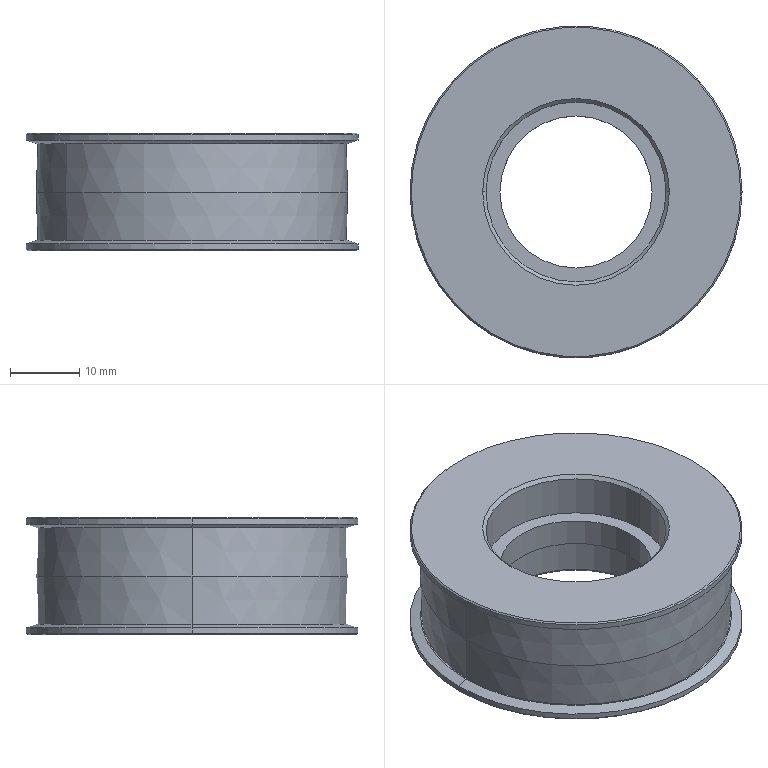Part | NX | features BREP 1 | 1 solid | 32 faces | box 48 x 48 x 17 mm | volume 18937 mm3 | cone 16 | cylinder 10 | plane 6 | commonest cylinder face diameters 26 x4 48 x4 22 x2
STEP:
#1=CARTESIAN_POINT('',(23.8,0.,8.5));
#2=VERTEX_POINT('',#1);
#3=CARTESIAN_POINT('',(-23.8,0.,8.5));
#4=VERTEX_POINT('',#3);
#5=CARTESIAN_POINT('',(0.,0.,8.5));
#6=DIRECTION('',(0.,0.,1.));
#7=DIRECTION('',(1.,0.,0.));
#8=AXIS2_PLACEMENT_3D('',#5,#6,#7);
#9=CIRCLE('',#8,23.8);
#10=EDGE_CURVE('',#2,#4,#9,.T.);
#11=ORIENTED_EDGE('',*,*,#10,.F.);
#12=CARTESIAN_POINT('',(24.,0.,8.3));
#13=VERTEX_POINT('',#12);
#14=CARTESIAN_POINT('',(24.,0.,8.3));
#15=DIRECTION('',(0.7071,0.,-0.7071));
#16=VECTOR('',#15,1000.);
#17=LINE('',#14,#16);
#18=EDGE_CURVE('',#2,#13,#17,.T.);
#19=ORIENTED_EDGE('',*,*,#18,.T.);
#20=CARTESIAN_POINT('',(-24.,0.,8.3));
#21=VERTEX_POINT('',#20);
#22=CARTESIAN_POINT('',(0.,0.,8.3));
#23=DIRECTION('',(0.,0.,-1.));
#24=DIRECTION('',(1.,0.,0.));
#25=AXIS2_PLACEMENT_3D('',#22,#23,#24);
#26=CIRCLE('',#25,24.);
#27=EDGE_CURVE('',#21,#13,#26,.T.);
#28=ORIENTED_EDGE('',*,*,#27,.F.);
#29=CARTESIAN_POINT('',(-24.,0.,8.3));
#30=DIRECTION('',(-0.7071,0.,-0.7071));
#31=VECTOR('',#30,1000.);
#32=LINE('',#29,#31);
#33=EDGE_CURVE('',#4,#21,#32,.T.);
#34=ORIENTED_EDGE('',*,*,#33,.F.);
#35=EDGE_LOOP('',(#11,#19,#28,#34));
#36=FACE_BOUND('',#35,.T.);
#37=CARTESIAN_POINT('',(0.,0.,8.3));
#38=DIRECTION('',(0.,0.,-1.));
#39=DIRECTION('',(-1.,0.,0.));
#40=AXIS2_PLACEMENT_3D('',#37,#38,#39);
#41=CONICAL_SURFACE('',#40,24.,0.7854);
#42=ADVANCED_FACE('',(#36),#41,.T.);
#43=CARTESIAN_POINT('',(-23.8,0.,-8.5));
#44=VERTEX_POINT('',#43);
#45=CARTESIAN_POINT('',(23.8,0.,-8.5));
#46=VERTEX_POINT('',#45);
#47=CARTESIAN_POINT('',(0.,0.,-8.5));
#48=DIRECTION('',(0.,0.,-1.));
#49=DIRECTION('',(1.,0.,0.));
#50=AXIS2_PLACEMENT_3D('',#47,#48,#49);
#51=CIRCLE('',#50,23.8);
#52=EDGE_CURVE('',#44,#46,#51,.T.);
#53=ORIENTED_EDGE('',*,*,#52,.F.);
#54=CARTESIAN_POINT('',(-24.,0.,-8.3));
#55=VERTEX_POINT('',#54);
#56=CARTESIAN_POINT('',(-23.8,0.,-8.5));
#57=DIRECTION('',(-0.7071,0.,0.7071));
#58=VECTOR('',#57,1000.);
#59=LINE('',#56,#58);
#60=EDGE_CURVE('',#55,#44,#59,.F.);
#61=ORIENTED_EDGE('',*,*,#60,.F.);
#62=CARTESIAN_POINT('',(24.,0.,-8.3));
#63=VERTEX_POINT('',#62);
#64=CARTESIAN_POINT('',(0.,0.,-8.3));
#65=DIRECTION('',(0.,0.,1.));
#66=DIRECTION('',(1.,0.,0.));
#67=AXIS2_PLACEMENT_3D('',#64,#65,#66);
#68=CIRCLE('',#67,24.);
#69=EDGE_CURVE('',#63,#55,#68,.T.);
#70=ORIENTED_EDGE('',*,*,#69,.F.);
#71=CARTESIAN_POINT('',(23.8,0.,-8.5));
#72=DIRECTION('',(0.7071,0.,0.7071));
#73=VECTOR('',#72,1000.);
#74=LINE('',#71,#73);
#75=EDGE_CURVE('',#63,#46,#74,.F.);
#76=ORIENTED_EDGE('',*,*,#75,.T.);
#77=EDGE_LOOP('',(#53,#61,#70,#76));
#78=FACE_BOUND('',#77,.T.);
#79=CARTESIAN_POINT('',(0.,0.,-8.5));
#80=DIRECTION('',(0.,0.,1.));
#81=DIRECTION('',(1.,0.,0.));
#82=AXIS2_PLACEMENT_3D('',#79,#80,#81);
#83=CONICAL_SURFACE('',#82,23.8,0.7854);
#84=ADVANCED_FACE('',(#78),#83,.T.);
#85=CARTESIAN_POINT('',(-13.,0.,8.));
#86=VERTEX_POINT('',#85);
#87=CARTESIAN_POINT('',(13.,0.,8.));
#88=VERTEX_POINT('',#87);
#89=CARTESIAN_POINT('',(0.,0.,8.));
#90=DIRECTION('',(0.,0.,1.));
#91=DIRECTION('',(1.,0.,0.));
#92=AXIS2_PLACEMENT_3D('',#89,#90,#91);
#93=CIRCLE('',#92,13.);
#94=EDGE_CURVE('',#86,#88,#93,.T.);
#95=ORIENTED_EDGE('',*,*,#94,.F.);
#96=CARTESIAN_POINT('',(-13.5,0.,8.5));
#97=VERTEX_POINT('',#96);
#98=CARTESIAN_POINT('',(-13.,0.,8.));
#99=DIRECTION('',(-0.7071,0.,0.7071));
#100=VECTOR('',#99,1000.);
#101=LINE('',#98,#100);
#102=EDGE_CURVE('',#97,#86,#101,.F.);
#103=ORIENTED_EDGE('',*,*,#102,.F.);
#104=CARTESIAN_POINT('',(13.5,0.,8.5));
#105=VERTEX_POINT('',#104);
#106=CARTESIAN_POINT('',(0.,0.,8.5));
#107=DIRECTION('',(0.,0.,-1.));
#108=DIRECTION('',(1.,0.,0.));
#109=AXIS2_PLACEMENT_3D('',#106,#107,#108);
#110=CIRCLE('',#109,13.5);
#111=EDGE_CURVE('',#105,#97,#110,.T.);
#112=ORIENTED_EDGE('',*,*,#111,.F.);
#113=CARTESIAN_POINT('',(13.,0.,8.));
#114=DIRECTION('',(0.7071,0.,0.7071));
#115=VECTOR('',#114,1000.);
#116=LINE('',#113,#115);
#117=EDGE_CURVE('',#105,#88,#116,.F.);
#118=ORIENTED_EDGE('',*,*,#117,.T.);
#119=EDGE_LOOP('',(#95,#103,#112,#118));
#120=FACE_BOUND('',#119,.T.);
#121=CARTESIAN_POINT('',(0.,0.,8.));
#122=DIRECTION('',(0.,0.,1.));
#123=DIRECTION('',(1.,0.,0.));
#124=AXIS2_PLACEMENT_3D('',#121,#122,#123);
#125=CONICAL_SURFACE('',#124,13.,0.7854);
#126=ADVANCED_FACE('',(#120),#125,.F.);
#127=CARTESIAN_POINT('',(13.,0.,-8.));
#128=VERTEX_POINT('',#127);
#129=CARTESIAN_POINT('',(-13.,0.,-8.));
#130=VERTEX_POINT('',#129);
#131=CARTESIAN_POINT('',(0.,0.,-8.));
#132=DIRECTION('',(0.,0.,-1.));
#133=DIRECTION('',(1.,0.,0.));
#134=AXIS2_PLACEMENT_3D('',#131,#132,#133);
#135=CIRCLE('',#134,13.);
#136=EDGE_CURVE('',#128,#130,#135,.T.);
#137=ORIENTED_EDGE('',*,*,#136,.F.);
#138=CARTESIAN_POINT('',(13.5,0.,-8.5));
#139=VERTEX_POINT('',#138);
#140=CARTESIAN_POINT('',(13.,0.,-8.));
#141=DIRECTION('',(0.7071,0.,-0.7071));
#142=VECTOR('',#141,1000.);
#143=LINE('',#140,#142);
#144=EDGE_CURVE('',#128,#139,#143,.T.);
#145=ORIENTED_EDGE('',*,*,#144,.T.);
#146=CARTESIAN_POINT('',(-13.5,0.,-8.5));
#147=VERTEX_POINT('',#146);
#148=CARTESIAN_POINT('',(0.,0.,-8.5));
#149=DIRECTION('',(0.,0.,1.));
#150=DIRECTION('',(1.,0.,0.));
#151=AXIS2_PLACEMENT_3D('',#148,#149,#150);
#152=CIRCLE('',#151,13.5);
#153=EDGE_CURVE('',#147,#139,#152,.T.);
#154=ORIENTED_EDGE('',*,*,#153,.F.);
#155=CARTESIAN_POINT('',(-13.,0.,-8.));
#156=DIRECTION('',(-0.7071,0.,-0.7071));
#157=VECTOR('',#156,1000.);
#158=LINE('',#155,#157);
#159=EDGE_CURVE('',#130,#147,#158,.T.);
#160=ORIENTED_EDGE('',*,*,#159,.F.);
#161=EDGE_LOOP('',(#137,#145,#154,#160));
#162=FACE_BOUND('',#161,.T.);
#163=CARTESIAN_POINT('',(0.,0.,-8.));
#164=DIRECTION('',(0.,0.,-1.));
#165=DIRECTION('',(-1.,0.,0.));
#166=AXIS2_PLACEMENT_3D('',#163,#164,#165);
#167=CONICAL_SURFACE('',#166,13.,0.7854);
#168=ADVANCED_FACE('',(#162),#167,.F.);
#169=CARTESIAN_POINT('',(13.,0.,-2.));
#170=VERTEX_POINT('',#169);
#171=CARTESIAN_POINT('',(-13.,0.,-2.));
#172=VERTEX_POINT('',#171);
#173=CARTESIAN_POINT('',(0.,0.,-2.));
#174=DIRECTION('',(0.,0.,-1.));
#175=DIRECTION('',(-1.,0.,0.));
#176=AXIS2_PLACEMENT_3D('',#173,#174,#175);
#177=CIRCLE('',#176,13.);
#178=EDGE_CURVE('',#170,#172,#177,.T.);
#179=ORIENTED_EDGE('',*,*,#178,.F.);
#180=CARTESIAN_POINT('',(13.,0.,-2.));
#181=DIRECTION('',(0.,0.,-1.));
#182=VECTOR('',#181,1000.);
#183=LINE('',#180,#182);
#184=EDGE_CURVE('',#170,#128,#183,.T.);
#185=ORIENTED_EDGE('',*,*,#184,.T.);
#186=ORIENTED_EDGE('',*,*,#136,.T.);
#187=CARTESIAN_POINT('',(-13.,0.,-2.));
#188=DIRECTION('',(0.,0.,-1.));
#189=VECTOR('',#188,1000.);
#190=LINE('',#187,#189);
#191=EDGE_CURVE('',#172,#130,#190,.T.);
#192=ORIENTED_EDGE('',*,*,#191,.F.);
#193=EDGE_LOOP('',(#179,#185,#186,#192));
#194=FACE_BOUND('',#193,.T.);
#195=CARTESIAN_POINT('',(0.,0.,-2.));
#196=DIRECTION('',(0.,0.,-1.));
#197=DIRECTION('',(-1.,0.,0.));
#198=AXIS2_PLACEMENT_3D('',#195,#196,#197);
#199=CYLINDRICAL_SURFACE('',#198,13.);
#200=ADVANCED_FACE('',(#194),#199,.F.);
#201=CARTESIAN_POINT('',(-13.,0.,2.));
#202=VERTEX_POINT('',#201);
#203=CARTESIAN_POINT('',(13.,0.,2.));
#204=VERTEX_POINT('',#203);
#205=CARTESIAN_POINT('',(0.,0.,2.));
#206=DIRECTION('',(0.,0.,1.));
#207=DIRECTION('',(1.,0.,0.));
#208=AXIS2_PLACEMENT_3D('',#205,#206,#207);
#209=CIRCLE('',#208,13.);
#210=EDGE_CURVE('',#202,#204,#209,.T.);
#211=ORIENTED_EDGE('',*,*,#210,.F.);
#212=CARTESIAN_POINT('',(-13.,0.,2.));
#213=DIRECTION('',(0.,0.,1.));
#214=VECTOR('',#213,1000.);
#215=LINE('',#212,#214);
#216=EDGE_CURVE('',#86,#202,#215,.F.);
#217=ORIENTED_EDGE('',*,*,#216,.F.);
#218=ORIENTED_EDGE('',*,*,#94,.T.);
#219=CARTESIAN_POINT('',(13.,0.,2.));
#220=DIRECTION('',(0.,0.,1.));
#221=VECTOR('',#220,1000.);
#222=LINE('',#219,#221);
#223=EDGE_CURVE('',#88,#204,#222,.F.);
#224=ORIENTED_EDGE('',*,*,#223,.T.);
#225=EDGE_LOOP('',(#211,#217,#218,#224));
#226=FACE_BOUND('',#225,.T.);
#227=CARTESIAN_POINT('',(0.,0.,2.));
#228=DIRECTION('',(0.,0.,1.));
#229=DIRECTION('',(1.,0.,0.));
#230=AXIS2_PLACEMENT_3D('',#227,#228,#229);
#231=CYLINDRICAL_SURFACE('',#230,13.);
#232=ADVANCED_FACE('',(#226),#231,.F.);
#233=CARTESIAN_POINT('',(22.5,0.,-7.));
#234=VERTEX_POINT('',#233);
#235=CARTESIAN_POINT('',(-22.5,0.,-7.));
#236=VERTEX_POINT('',#235);
#237=CARTESIAN_POINT('',(0.,0.,-7.));
#238=DIRECTION('',(0.,0.,-1.));
#239=DIRECTION('',(-1.,0.,0.));
#240=AXIS2_PLACEMENT_3D('',#237,#238,#239);
#241=CIRCLE('',#240,22.5);
#242=EDGE_CURVE('',#234,#236,#241,.T.);
#243=ORIENTED_EDGE('',*,*,#242,.T.);
#244=CARTESIAN_POINT('',(-24.,0.,-7.5));
#245=VERTEX_POINT('',#244);
#246=CARTESIAN_POINT('',(-22.5,0.,-7.));
#247=DIRECTION('',(-0.9487,0.,-0.3162));
#248=VECTOR('',#247,1000.);
#249=LINE('',#246,#248);
#250=EDGE_CURVE('',#245,#236,#249,.F.);
#251=ORIENTED_EDGE('',*,*,#250,.F.);
#252=CARTESIAN_POINT('',(24.,0.,-7.5));
#253=VERTEX_POINT('',#252);
#254=CARTESIAN_POINT('',(0.,0.,-7.5));
#255=DIRECTION('',(0.,0.,-1.));
#256=DIRECTION('',(-1.,0.,0.));
#257=AXIS2_PLACEMENT_3D('',#254,#255,#256);
#258=CIRCLE('',#257,24.);
#259=EDGE_CURVE('',#253,#245,#258,.T.);
#260=ORIENTED_EDGE('',*,*,#259,.F.);
#261=CARTESIAN_POINT('',(22.5,0.,-7.));
#262=DIRECTION('',(0.9487,0.,-0.3162));
#263=VECTOR('',#262,1000.);
#264=LINE('',#261,#263);
#265=EDGE_CURVE('',#253,#234,#264,.F.);
#266=ORIENTED_EDGE('',*,*,#265,.T.);
#267=EDGE_LOOP('',(#243,#251,#260,#266));
#268=FACE_BOUND('',#267,.T.);
#269=CARTESIAN_POINT('',(0.,0.,-7.));
#270=DIRECTION('',(0.,0.,-1.));
#271=DIRECTION('',(1.,0.,0.));
#272=AXIS2_PLACEMENT_3D('',#269,#270,#271);
#273=CONICAL_SURFACE('',#272,22.5,1.249);
#274=ADVANCED_FACE('',(#268),#273,.T.);
#275=CARTESIAN_POINT('',(0.,0.,-8.3));
#276=DIRECTION('',(0.,0.,1.));
#277=DIRECTION('',(1.,0.,0.));
#278=AXIS2_PLACEMENT_3D('',#275,#276,#277);
#279=CIRCLE('',#278,24.);
#280=EDGE_CURVE('',#55,#63,#279,.T.);
#281=ORIENTED_EDGE('',*,*,#280,.T.);
#282=CARTESIAN_POINT('',(24.,0.,0.));
#283=DIRECTION('',(0.,0.,1.));
#284=VECTOR('',#283,1000.);
#285=LINE('',#282,#284);
#286=EDGE_CURVE('',#63,#253,#285,.T.);
#287=ORIENTED_EDGE('',*,*,#286,.T.);
#288=ORIENTED_EDGE('',*,*,#259,.T.);
#289=CARTESIAN_POINT('',(-24.,0.,0.));
#290=DIRECTION('',(0.,0.,1.));
#291=VECTOR('',#290,1000.);
#292=LINE('',#289,#291);
#293=EDGE_CURVE('',#55,#245,#292,.T.);
#294=ORIENTED_EDGE('',*,*,#293,.F.);
#295=EDGE_LOOP('',(#281,#287,#288,#294));
#296=FACE_BOUND('',#295,.T.);
#297=CARTESIAN_POINT('',(0.,0.,0.));
#298=DIRECTION('',(0.,0.,1.));
#299=DIRECTION('',(-1.,0.,0.));
#300=AXIS2_PLACEMENT_3D('',#297,#298,#299);
#301=CYLINDRICAL_SURFACE('',#300,24.);
#302=ADVANCED_FACE('',(#296),#301,.T.);
#303=CARTESIAN_POINT('',(22.3,0.,-7.));
#304=VERTEX_POINT('',#303);
#305=CARTESIAN_POINT('',(-22.3,0.,-7.));
#306=VERTEX_POINT('',#305);
#307=CARTESIAN_POINT('',(0.,0.,-7.));
#308=DIRECTION('',(0.,0.,-1.));
#309=DIRECTION('',(-1.,0.,0.));
#310=AXIS2_PLACEMENT_3D('',#307,#308,#309);
#311=CIRCLE('',#310,22.3);
#312=EDGE_CURVE('',#304,#306,#311,.T.);
#313=ORIENTED_EDGE('',*,*,#312,.F.);
#314=CARTESIAN_POINT('',(22.5,0.,0.));
#315=VERTEX_POINT('',#314);
#316=CARTESIAN_POINT('',(22.3,0.,-7.));
#317=DIRECTION('',(0.02856,0.,0.9996));
#318=VECTOR('',#317,1000.);
#319=LINE('',#316,#318);
#320=EDGE_CURVE('',#304,#315,#319,.T.);
#321=ORIENTED_EDGE('',*,*,#320,.T.);
#322=CARTESIAN_POINT('',(-22.5,0.,0.));
#323=VERTEX_POINT('',#322);
#324=CARTESIAN_POINT('',(0.,0.,0.));
#325=DIRECTION('',(0.,0.,-1.));
#326=DIRECTION('',(-1.,0.,0.));
#327=AXIS2_PLACEMENT_3D('',#324,#325,#326);
#328=CIRCLE('',#327,22.5);
#329=EDGE_CURVE('',#315,#323,#328,.T.);
#330=ORIENTED_EDGE('',*,*,#329,.T.);
#331=CARTESIAN_POINT('',(-22.3,0.,-7.));
#332=DIRECTION('',(-0.02856,0.,0.9996));
#333=VECTOR('',#332,1000.);
#334=LINE('',#331,#333);
#335=EDGE_CURVE('',#306,#323,#334,.T.);
#336=ORIENTED_EDGE('',*,*,#335,.F.);
#337=EDGE_LOOP('',(#313,#321,#330,#336));
#338=FACE_BOUND('',#337,.T.);
#339=CARTESIAN_POINT('',(0.,0.,-7.));
#340=DIRECTION('',(0.,0.,1.));
#341=DIRECTION('',(-1.,0.,0.));
#342=AXIS2_PLACEMENT_3D('',#339,#340,#341);
#343=CONICAL_SURFACE('',#342,22.3,0.02856);
#344=ADVANCED_FACE('',(#338),#343,.T.);
#345=CARTESIAN_POINT('',(-22.5,0.,7.));
#346=VERTEX_POINT('',#345);
#347=CARTESIAN_POINT('',(22.5,0.,7.));
#348=VERTEX_POINT('',#347);
#349=CARTESIAN_POINT('',(0.,0.,7.));
#350=DIRECTION('',(0.,0.,-1.));
#351=DIRECTION('',(-1.,0.,0.));
#352=AXIS2_PLACEMENT_3D('',#349,#350,#351);
#353=CIRCLE('',#352,22.5);
#354=EDGE_CURVE('',#346,#348,#353,.T.);
#355=ORIENTED_EDGE('',*,*,#354,.F.);
#356=CARTESIAN_POINT('',(-24.,0.,7.5));
#357=VERTEX_POINT('',#356);
#358=CARTESIAN_POINT('',(-22.5,0.,7.));
#359=DIRECTION('',(-0.9487,0.,0.3162));
#360=VECTOR('',#359,1000.);
#361=LINE('',#358,#360);
#362=EDGE_CURVE('',#357,#346,#361,.F.);
#363=ORIENTED_EDGE('',*,*,#362,.F.);
#364=CARTESIAN_POINT('',(24.,0.,7.5));
#365=VERTEX_POINT('',#364);
#366=CARTESIAN_POINT('',(0.,0.,7.5));
#367=DIRECTION('',(0.,0.,-1.));
#368=DIRECTION('',(-1.,0.,0.));
#369=AXIS2_PLACEMENT_3D('',#366,#367,#368);
#370=CIRCLE('',#369,24.);
#371=EDGE_CURVE('',#357,#365,#370,.T.);
#372=ORIENTED_EDGE('',*,*,#371,.T.);
#373=CARTESIAN_POINT('',(22.5,0.,7.));
#374=DIRECTION('',(0.9487,0.,0.3162));
#375=VECTOR('',#374,1000.);
#376=LINE('',#373,#375);
#377=EDGE_CURVE('',#365,#348,#376,.F.);
#378=ORIENTED_EDGE('',*,*,#377,.T.);
#379=EDGE_LOOP('',(#355,#363,#372,#378));
#380=FACE_BOUND('',#379,.T.);
#381=CARTESIAN_POINT('',(0.,0.,7.));
#382=DIRECTION('',(0.,0.,1.));
#383=DIRECTION('',(1.,0.,0.));
#384=AXIS2_PLACEMENT_3D('',#381,#382,#383);
#385=CONICAL_SURFACE('',#384,22.5,1.249);
#386=ADVANCED_FACE('',(#380),#385,.T.);
#387=ORIENTED_EDGE('',*,*,#27,.T.);
#388=CARTESIAN_POINT('',(24.,0.,0.));
#389=DIRECTION('',(0.,0.,-1.));
#390=VECTOR('',#389,1000.);
#391=LINE('',#388,#390);
#392=EDGE_CURVE('',#13,#365,#391,.T.);
#393=ORIENTED_EDGE('',*,*,#392,.T.);
#394=ORIENTED_EDGE('',*,*,#371,.F.);
#395=CARTESIAN_POINT('',(-24.,0.,0.));
#396=DIRECTION('',(0.,0.,-1.));
#397=VECTOR('',#396,1000.);
#398=LINE('',#395,#397);
#399=EDGE_CURVE('',#21,#357,#398,.T.);
#400=ORIENTED_EDGE('',*,*,#399,.F.);
#401=EDGE_LOOP('',(#387,#393,#394,#400));
#402=FACE_BOUND('',#401,.T.);
#403=CARTESIAN_POINT('',(0.,0.,0.));
#404=DIRECTION('',(0.,0.,-1.));
#405=DIRECTION('',(-1.,0.,0.));
#406=AXIS2_PLACEMENT_3D('',#403,#404,#405);
#407=CYLINDRICAL_SURFACE('',#406,24.);
#408=ADVANCED_FACE('',(#402),#407,.T.);
#409=CARTESIAN_POINT('',(-22.3,0.,7.));
#410=VERTEX_POINT('',#409);
#411=CARTESIAN_POINT('',(22.3,0.,7.));
#412=VERTEX_POINT('',#411);
#413=CARTESIAN_POINT('',(0.,0.,7.));
#414=DIRECTION('',(0.,0.,-1.));
#415=DIRECTION('',(-1.,0.,0.));
#416=AXIS2_PLACEMENT_3D('',#413,#414,#415);
#417=CIRCLE('',#416,22.3);
#418=EDGE_CURVE('',#410,#412,#417,.T.);
#419=ORIENTED_EDGE('',*,*,#418,.T.);
#420=CARTESIAN_POINT('',(22.3,0.,7.));
#421=DIRECTION('',(0.02856,0.,-0.9996));
#422=VECTOR('',#421,1000.);
#423=LINE('',#420,#422);
#424=EDGE_CURVE('',#412,#315,#423,.T.);
#425=ORIENTED_EDGE('',*,*,#424,.T.);
#426=CARTESIAN_POINT('',(0.,0.,0.));
#427=DIRECTION('',(0.,0.,-1.));
#428=DIRECTION('',(-1.,0.,0.));
#429=AXIS2_PLACEMENT_3D('',#426,#427,#428);
#430=CIRCLE('',#429,22.5);
#431=EDGE_CURVE('',#323,#315,#430,.T.);
#432=ORIENTED_EDGE('',*,*,#431,.F.);
#433=CARTESIAN_POINT('',(-22.3,0.,7.));
#434=DIRECTION('',(-0.02856,0.,-0.9996));
#435=VECTOR('',#434,1000.);
#436=LINE('',#433,#435);
#437=EDGE_CURVE('',#410,#323,#436,.T.);
#438=ORIENTED_EDGE('',*,*,#437,.F.);
#439=EDGE_LOOP('',(#419,#425,#432,#438));
#440=FACE_BOUND('',#439,.T.);
#441=CARTESIAN_POINT('',(0.,0.,7.));
#442=DIRECTION('',(0.,0.,-1.));
#443=DIRECTION('',(-1.,0.,0.));
#444=AXIS2_PLACEMENT_3D('',#441,#442,#443);
#445=CONICAL_SURFACE('',#444,22.3,0.02856);
#446=ADVANCED_FACE('',(#440),#445,.T.);
#447=CARTESIAN_POINT('',(-11.,0.,-2.));
#448=VERTEX_POINT('',#447);
#449=CARTESIAN_POINT('',(11.,0.,-2.));
#450=VERTEX_POINT('',#449);
#451=CARTESIAN_POINT('',(0.,0.,-2.));
#452=DIRECTION('',(0.,0.,1.));
#453=DIRECTION('',(-1.,0.,0.));
#454=AXIS2_PLACEMENT_3D('',#451,#452,#453);
#455=CIRCLE('',#454,11.);
#456=EDGE_CURVE('',#448,#450,#455,.T.);
#457=ORIENTED_EDGE('',*,*,#456,.F.);
#458=CARTESIAN_POINT('',(-11.,0.,2.));
#459=VERTEX_POINT('',#458);
#460=CARTESIAN_POINT('',(-11.,0.,-19.));
#461=DIRECTION('',(0.,0.,1.));
#462=VECTOR('',#461,1000.);
#463=LINE('',#460,#462);
#464=EDGE_CURVE('',#459,#448,#463,.F.);
#465=ORIENTED_EDGE('',*,*,#464,.F.);
#466=CARTESIAN_POINT('',(11.,0.,2.));
#467=VERTEX_POINT('',#466);
#468=CARTESIAN_POINT('',(0.,0.,2.));
#469=DIRECTION('',(0.,0.,1.));
#470=DIRECTION('',(1.,0.,0.));
#471=AXIS2_PLACEMENT_3D('',#468,#469,#470);
#472=CIRCLE('',#471,11.);
#473=EDGE_CURVE('',#459,#467,#472,.T.);
#474=ORIENTED_EDGE('',*,*,#473,.T.);
#475=CARTESIAN_POINT('',(11.,0.,-19.));
#476=DIRECTION('',(0.,0.,1.));
#477=VECTOR('',#476,1000.);
#478=LINE('',#475,#477);
#479=EDGE_CURVE('',#467,#450,#478,.F.);
#480=ORIENTED_EDGE('',*,*,#479,.T.);
#481=EDGE_LOOP('',(#457,#465,#474,#480));
#482=FACE_BOUND('',#481,.T.);
#483=CARTESIAN_POINT('',(0.,0.,-19.));
#484=DIRECTION('',(0.,0.,1.));
#485=DIRECTION('',(1.,0.,0.));
#486=AXIS2_PLACEMENT_3D('',#483,#484,#485);
#487=CYLINDRICAL_SURFACE('',#486,11.);
#488=ADVANCED_FACE('',(#482),#487,.F.);
#489=ORIENTED_EDGE('',*,*,#464,.T.);
#490=CARTESIAN_POINT('',(0.,0.,-2.));
#491=DIRECTION('',(0.,0.,1.));
#492=DIRECTION('',(-1.,0.,0.));
#493=AXIS2_PLACEMENT_3D('',#490,#491,#492);
#494=CIRCLE('',#493,11.);
#495=EDGE_CURVE('',#450,#448,#494,.T.);
#496=ORIENTED_EDGE('',*,*,#495,.F.);
#497=ORIENTED_EDGE('',*,*,#479,.F.);
#498=CARTESIAN_POINT('',(0.,0.,2.));
#499=DIRECTION('',(0.,0.,1.));
#500=DIRECTION('',(1.,0.,0.));
#501=AXIS2_PLACEMENT_3D('',#498,#499,#500);
#502=CIRCLE('',#501,11.);
#503=EDGE_CURVE('',#467,#459,#502,.T.);
#504=ORIENTED_EDGE('',*,*,#503,.T.);
#505=EDGE_LOOP('',(#489,#496,#497,#504));
#506=FACE_BOUND('',#505,.T.);
#507=CARTESIAN_POINT('',(0.,0.,-19.));
#508=DIRECTION('',(0.,0.,1.));
#509=DIRECTION('',(1.,0.,0.));
#510=AXIS2_PLACEMENT_3D('',#507,#508,#509);
#511=CYLINDRICAL_SURFACE('',#510,11.);
#512=ADVANCED_FACE('',(#506),#511,.F.);
#513=CARTESIAN_POINT('',(0.,0.,7.));
#514=DIRECTION('',(0.,0.,-1.));
#515=DIRECTION('',(-1.,0.,0.));
#516=AXIS2_PLACEMENT_3D('',#513,#514,#515);
#517=CIRCLE('',#516,22.5);
#518=EDGE_CURVE('',#348,#346,#517,.T.);
#519=ORIENTED_EDGE('',*,*,#518,.T.);
#520=ORIENTED_EDGE('',*,*,#354,.T.);
#521=EDGE_LOOP('',(#519,#520));
#522=FACE_BOUND('',#521,.T.);
#523=ORIENTED_EDGE('',*,*,#418,.F.);
#524=CARTESIAN_POINT('',(0.,0.,7.));
#525=DIRECTION('',(0.,0.,-1.));
#526=DIRECTION('',(-1.,0.,0.));
#527=AXIS2_PLACEMENT_3D('',#524,#525,#526);
#528=CIRCLE('',#527,22.3);
#529=EDGE_CURVE('',#412,#410,#528,.T.);
#530=ORIENTED_EDGE('',*,*,#529,.F.);
#531=EDGE_LOOP('',(#523,#530));
#532=FACE_BOUND('',#531,.T.);
#533=CARTESIAN_POINT('',(-22.5,0.,7.));
#534=DIRECTION('',(0.,0.,1.));
#535=DIRECTION('',(1.,0.,0.));
#536=AXIS2_PLACEMENT_3D('',#533,#534,#535);
#537=PLANE('',#536);
#538=ADVANCED_FACE('',(#522,#532),#537,.F.);
#539=ORIENTED_EDGE('',*,*,#424,.F.);
#540=ORIENTED_EDGE('',*,*,#529,.T.);
#541=ORIENTED_EDGE('',*,*,#437,.T.);
#542=ORIENTED_EDGE('',*,*,#329,.F.);
#543=EDGE_LOOP('',(#539,#540,#541,#542));
#544=FACE_BOUND('',#543,.T.);
#545=CARTESIAN_POINT('',(0.,0.,7.));
#546=DIRECTION('',(0.,0.,-1.));
#547=DIRECTION('',(-1.,0.,0.));
#548=AXIS2_PLACEMENT_3D('',#545,#546,#547);
#549=CONICAL_SURFACE('',#548,22.3,0.02856);
#550=ADVANCED_FACE('',(#544),#549,.T.);
#551=CARTESIAN_POINT('',(0.,0.,8.5));
#552=DIRECTION('',(0.,0.,1.));
#553=DIRECTION('',(1.,0.,0.));
#554=AXIS2_PLACEMENT_3D('',#551,#552,#553);
#555=CIRCLE('',#554,23.8);
#556=EDGE_CURVE('',#4,#2,#555,.T.);
#557=ORIENTED_EDGE('',*,*,#556,.T.);
#558=ORIENTED_EDGE('',*,*,#10,.T.);
#559=EDGE_LOOP('',(#557,#558));
#560=FACE_BOUND('',#559,.T.);
#561=ORIENTED_EDGE('',*,*,#111,.T.);
#562=CARTESIAN_POINT('',(0.,0.,8.5));
#563=DIRECTION('',(0.,0.,-1.));
#564=DIRECTION('',(1.,0.,0.));
#565=AXIS2_PLACEMENT_3D('',#562,#563,#564);
#566=CIRCLE('',#565,13.5);
#567=EDGE_CURVE('',#97,#105,#566,.T.);
#568=ORIENTED_EDGE('',*,*,#567,.T.);
#569=EDGE_LOOP('',(#561,#568));
#570=FACE_BOUND('',#569,.T.);
#571=CARTESIAN_POINT('',(0.,0.,8.5));
#572=DIRECTION('',(0.,0.,1.));
#573=DIRECTION('',(1.,0.,0.));
#574=AXIS2_PLACEMENT_3D('',#571,#572,#573);
#575=PLANE('',#574);
#576=ADVANCED_FACE('',(#560,#570),#575,.T.);
#577=ORIENTED_EDGE('',*,*,#392,.F.);
#578=CARTESIAN_POINT('',(0.,0.,8.3));
#579=DIRECTION('',(0.,0.,-1.));
#580=DIRECTION('',(1.,0.,0.));
#581=AXIS2_PLACEMENT_3D('',#578,#579,#580);
#582=CIRCLE('',#581,24.);
#583=EDGE_CURVE('',#13,#21,#582,.T.);
#584=ORIENTED_EDGE('',*,*,#583,.T.);
#585=ORIENTED_EDGE('',*,*,#399,.T.);
#586=CARTESIAN_POINT('',(0.,0.,7.5));
#587=DIRECTION('',(0.,0.,-1.));
#588=DIRECTION('',(-1.,0.,0.));
#589=AXIS2_PLACEMENT_3D('',#586,#587,#588);
#590=CIRCLE('',#589,24.);
#591=EDGE_CURVE('',#365,#357,#590,.T.);
#592=ORIENTED_EDGE('',*,*,#591,.F.);
#593=EDGE_LOOP('',(#577,#584,#585,#592));
#594=FACE_BOUND('',#593,.T.);
#595=CARTESIAN_POINT('',(0.,0.,0.));
#596=DIRECTION('',(0.,0.,-1.));
#597=DIRECTION('',(-1.,0.,0.));
#598=AXIS2_PLACEMENT_3D('',#595,#596,#597);
#599=CYLINDRICAL_SURFACE('',#598,24.);
#600=ADVANCED_FACE('',(#594),#599,.T.);
#601=ORIENTED_EDGE('',*,*,#362,.T.);
#602=ORIENTED_EDGE('',*,*,#518,.F.);
#603=ORIENTED_EDGE('',*,*,#377,.F.);
#604=ORIENTED_EDGE('',*,*,#591,.T.);
#605=EDGE_LOOP('',(#601,#602,#603,#604));
#606=FACE_BOUND('',#605,.T.);
#607=CARTESIAN_POINT('',(0.,0.,7.));
#608=DIRECTION('',(0.,0.,1.));
#609=DIRECTION('',(1.,0.,0.));
#610=AXIS2_PLACEMENT_3D('',#607,#608,#609);
#611=CONICAL_SURFACE('',#610,22.5,1.249);
#612=ADVANCED_FACE('',(#606),#611,.T.);
#613=ORIENTED_EDGE('',*,*,#242,.F.);
#614=CARTESIAN_POINT('',(0.,0.,-7.));
#615=DIRECTION('',(0.,0.,-1.));
#616=DIRECTION('',(-1.,0.,0.));
#617=AXIS2_PLACEMENT_3D('',#614,#615,#616);
#618=CIRCLE('',#617,22.5);
#619=EDGE_CURVE('',#236,#234,#618,.T.);
#620=ORIENTED_EDGE('',*,*,#619,.F.);
#621=EDGE_LOOP('',(#613,#620));
#622=FACE_BOUND('',#621,.T.);
#623=CARTESIAN_POINT('',(0.,0.,-7.));
#624=DIRECTION('',(0.,0.,-1.));
#625=DIRECTION('',(-1.,0.,0.));
#626=AXIS2_PLACEMENT_3D('',#623,#624,#625);
#627=CIRCLE('',#626,22.3);
#628=EDGE_CURVE('',#306,#304,#627,.T.);
#629=ORIENTED_EDGE('',*,*,#628,.T.);
#630=ORIENTED_EDGE('',*,*,#312,.T.);
#631=EDGE_LOOP('',(#629,#630));
#632=FACE_BOUND('',#631,.T.);
#633=CARTESIAN_POINT('',(-22.5,0.,-7.));
#634=DIRECTION('',(0.,0.,-1.));
#635=DIRECTION('',(0.,-1.,0.));
#636=AXIS2_PLACEMENT_3D('',#633,#634,#635);
#637=PLANE('',#636);
#638=ADVANCED_FACE('',(#622,#632),#637,.F.);
#639=ORIENTED_EDGE('',*,*,#320,.F.);
#640=ORIENTED_EDGE('',*,*,#628,.F.);
#641=ORIENTED_EDGE('',*,*,#335,.T.);
#642=ORIENTED_EDGE('',*,*,#431,.T.);
#643=EDGE_LOOP('',(#639,#640,#641,#642));
#644=FACE_BOUND('',#643,.T.);
#645=CARTESIAN_POINT('',(0.,0.,-7.));
#646=DIRECTION('',(0.,0.,1.));
#647=DIRECTION('',(-1.,0.,0.));
#648=AXIS2_PLACEMENT_3D('',#645,#646,#647);
#649=CONICAL_SURFACE('',#648,22.3,0.02856);
#650=ADVANCED_FACE('',(#644),#649,.T.);
#651=CARTESIAN_POINT('',(0.,0.,-8.5));
#652=DIRECTION('',(0.,0.,-1.));
#653=DIRECTION('',(1.,0.,0.));
#654=AXIS2_PLACEMENT_3D('',#651,#652,#653);
#655=CIRCLE('',#654,23.8);
#656=EDGE_CURVE('',#46,#44,#655,.T.);
#657=ORIENTED_EDGE('',*,*,#656,.T.);
#658=ORIENTED_EDGE('',*,*,#52,.T.);
#659=EDGE_LOOP('',(#657,#658));
#660=FACE_BOUND('',#659,.T.);
#661=ORIENTED_EDGE('',*,*,#153,.T.);
#662=CARTESIAN_POINT('',(0.,0.,-8.5));
#663=DIRECTION('',(0.,0.,1.));
#664=DIRECTION('',(1.,0.,0.));
#665=AXIS2_PLACEMENT_3D('',#662,#663,#664);
#666=CIRCLE('',#665,13.5);
#667=EDGE_CURVE('',#139,#147,#666,.T.);
#668=ORIENTED_EDGE('',*,*,#667,.T.);
#669=EDGE_LOOP('',(#661,#668));
#670=FACE_BOUND('',#669,.T.);
#671=CARTESIAN_POINT('',(0.,0.,-8.5));
#672=DIRECTION('',(0.,0.,1.));
#673=DIRECTION('',(1.,0.,0.));
#674=AXIS2_PLACEMENT_3D('',#671,#672,#673);
#675=PLANE('',#674);
#676=ADVANCED_FACE('',(#660,#670),#675,.F.);
#677=ORIENTED_EDGE('',*,*,#286,.F.);
#678=ORIENTED_EDGE('',*,*,#69,.T.);
#679=ORIENTED_EDGE('',*,*,#293,.T.);
#680=CARTESIAN_POINT('',(0.,0.,-7.5));
#681=DIRECTION('',(0.,0.,-1.));
#682=DIRECTION('',(-1.,0.,0.));
#683=AXIS2_PLACEMENT_3D('',#680,#681,#682);
#684=CIRCLE('',#683,24.);
#685=EDGE_CURVE('',#245,#253,#684,.T.);
#686=ORIENTED_EDGE('',*,*,#685,.T.);
#687=EDGE_LOOP('',(#677,#678,#679,#686));
#688=FACE_BOUND('',#687,.T.);
#689=CARTESIAN_POINT('',(0.,0.,0.));
#690=DIRECTION('',(0.,0.,1.));
#691=DIRECTION('',(-1.,0.,0.));
#692=AXIS2_PLACEMENT_3D('',#689,#690,#691);
#693=CYLINDRICAL_SURFACE('',#692,24.);
#694=ADVANCED_FACE('',(#688),#693,.T.);
#695=ORIENTED_EDGE('',*,*,#250,.T.);
#696=ORIENTED_EDGE('',*,*,#619,.T.);
#697=ORIENTED_EDGE('',*,*,#265,.F.);
#698=ORIENTED_EDGE('',*,*,#685,.F.);
#699=EDGE_LOOP('',(#695,#696,#697,#698));
#700=FACE_BOUND('',#699,.T.);
#701=CARTESIAN_POINT('',(0.,0.,-7.));
#702=DIRECTION('',(0.,0.,-1.));
#703=DIRECTION('',(1.,0.,0.));
#704=AXIS2_PLACEMENT_3D('',#701,#702,#703);
#705=CONICAL_SURFACE('',#704,22.5,1.249);
#706=ADVANCED_FACE('',(#700),#705,.T.);
#707=ORIENTED_EDGE('',*,*,#216,.T.);
#708=CARTESIAN_POINT('',(0.,0.,2.));
#709=DIRECTION('',(0.,0.,1.));
#710=DIRECTION('',(1.,0.,0.));
#711=AXIS2_PLACEMENT_3D('',#708,#709,#710);
#712=CIRCLE('',#711,13.);
#713=EDGE_CURVE('',#204,#202,#712,.T.);
#714=ORIENTED_EDGE('',*,*,#713,.F.);
#715=ORIENTED_EDGE('',*,*,#223,.F.);
#716=CARTESIAN_POINT('',(0.,0.,8.));
#717=DIRECTION('',(0.,0.,1.));
#718=DIRECTION('',(1.,0.,0.));
#719=AXIS2_PLACEMENT_3D('',#716,#717,#718);
#720=CIRCLE('',#719,13.);
#721=EDGE_CURVE('',#88,#86,#720,.T.);
#722=ORIENTED_EDGE('',*,*,#721,.T.);
#723=EDGE_LOOP('',(#707,#714,#715,#722));
#724=FACE_BOUND('',#723,.T.);
#725=CARTESIAN_POINT('',(0.,0.,2.));
#726=DIRECTION('',(0.,0.,1.));
#727=DIRECTION('',(1.,0.,0.));
#728=AXIS2_PLACEMENT_3D('',#725,#726,#727);
#729=CYLINDRICAL_SURFACE('',#728,13.);
#730=ADVANCED_FACE('',(#724),#729,.F.);
#731=ORIENTED_EDGE('',*,*,#713,.T.);
#732=ORIENTED_EDGE('',*,*,#210,.T.);
#733=EDGE_LOOP('',(#731,#732));
#734=FACE_BOUND('',#733,.T.);
#735=ORIENTED_EDGE('',*,*,#503,.F.);
#736=ORIENTED_EDGE('',*,*,#473,.F.);
#737=EDGE_LOOP('',(#735,#736));
#738=FACE_BOUND('',#737,.T.);
#739=CARTESIAN_POINT('',(0.,0.,2.));
#740=DIRECTION('',(0.,0.,1.));
#741=DIRECTION('',(1.,0.,0.));
#742=AXIS2_PLACEMENT_3D('',#739,#740,#741);
#743=PLANE('',#742);
#744=ADVANCED_FACE('',(#734,#738),#743,.T.);
#745=CARTESIAN_POINT('',(0.,0.,-2.));
#746=DIRECTION('',(0.,0.,-1.));
#747=DIRECTION('',(-1.,0.,0.));
#748=AXIS2_PLACEMENT_3D('',#745,#746,#747);
#749=CIRCLE('',#748,13.);
#750=EDGE_CURVE('',#172,#170,#749,.T.);
#751=ORIENTED_EDGE('',*,*,#750,.T.);
#752=ORIENTED_EDGE('',*,*,#178,.T.);
#753=EDGE_LOOP('',(#751,#752));
#754=FACE_BOUND('',#753,.T.);
#755=ORIENTED_EDGE('',*,*,#495,.T.);
#756=ORIENTED_EDGE('',*,*,#456,.T.);
#757=EDGE_LOOP('',(#755,#756));
#758=FACE_BOUND('',#757,.T.);
#759=CARTESIAN_POINT('',(0.,0.,-2.));
#760=DIRECTION('',(0.,0.,-1.));
#761=DIRECTION('',(0.,-1.,0.));
#762=AXIS2_PLACEMENT_3D('',#759,#760,#761);
#763=PLANE('',#762);
#764=ADVANCED_FACE('',(#754,#758),#763,.T.);
#765=ORIENTED_EDGE('',*,*,#184,.F.);
#766=ORIENTED_EDGE('',*,*,#750,.F.);
#767=ORIENTED_EDGE('',*,*,#191,.T.);
#768=CARTESIAN_POINT('',(0.,0.,-8.));
#769=DIRECTION('',(0.,0.,-1.));
#770=DIRECTION('',(1.,0.,0.));
#771=AXIS2_PLACEMENT_3D('',#768,#769,#770);
#772=CIRCLE('',#771,13.);
#773=EDGE_CURVE('',#130,#128,#772,.T.);
#774=ORIENTED_EDGE('',*,*,#773,.T.);
#775=EDGE_LOOP('',(#765,#766,#767,#774));
#776=FACE_BOUND('',#775,.T.);
#777=CARTESIAN_POINT('',(0.,0.,-2.));
#778=DIRECTION('',(0.,0.,-1.));
#779=DIRECTION('',(-1.,0.,0.));
#780=AXIS2_PLACEMENT_3D('',#777,#778,#779);
#781=CYLINDRICAL_SURFACE('',#780,13.);
#782=ADVANCED_FACE('',(#776),#781,.F.);
#783=ORIENTED_EDGE('',*,*,#144,.F.);
#784=ORIENTED_EDGE('',*,*,#773,.F.);
#785=ORIENTED_EDGE('',*,*,#159,.T.);
#786=ORIENTED_EDGE('',*,*,#667,.F.);
#787=EDGE_LOOP('',(#783,#784,#785,#786));
#788=FACE_BOUND('',#787,.T.);
#789=CARTESIAN_POINT('',(0.,0.,-8.));
#790=DIRECTION('',(0.,0.,-1.));
#791=DIRECTION('',(-1.,0.,0.));
#792=AXIS2_PLACEMENT_3D('',#789,#790,#791);
#793=CONICAL_SURFACE('',#792,13.,0.7854);
#794=ADVANCED_FACE('',(#788),#793,.F.);
#795=ORIENTED_EDGE('',*,*,#102,.T.);
#796=ORIENTED_EDGE('',*,*,#721,.F.);
#797=ORIENTED_EDGE('',*,*,#117,.F.);
#798=ORIENTED_EDGE('',*,*,#567,.F.);
#799=EDGE_LOOP('',(#795,#796,#797,#798));
#800=FACE_BOUND('',#799,.T.);
#801=CARTESIAN_POINT('',(0.,0.,8.));
#802=DIRECTION('',(0.,0.,1.));
#803=DIRECTION('',(1.,0.,0.));
#804=AXIS2_PLACEMENT_3D('',#801,#802,#803);
#805=CONICAL_SURFACE('',#804,13.,0.7854);
#806=ADVANCED_FACE('',(#800),#805,.F.);
#807=ORIENTED_EDGE('',*,*,#60,.T.);
#808=ORIENTED_EDGE('',*,*,#656,.F.);
#809=ORIENTED_EDGE('',*,*,#75,.F.);
#810=ORIENTED_EDGE('',*,*,#280,.F.);
#811=EDGE_LOOP('',(#807,#808,#809,#810));
#812=FACE_BOUND('',#811,.T.);
#813=CARTESIAN_POINT('',(0.,0.,-8.5));
#814=DIRECTION('',(0.,0.,1.));
#815=DIRECTION('',(1.,0.,0.));
#816=AXIS2_PLACEMENT_3D('',#813,#814,#815);
#817=CONICAL_SURFACE('',#816,23.8,0.7854);
#818=ADVANCED_FACE('',(#812),#817,.T.);
#819=ORIENTED_EDGE('',*,*,#18,.F.);
#820=ORIENTED_EDGE('',*,*,#556,.F.);
#821=ORIENTED_EDGE('',*,*,#33,.T.);
#822=ORIENTED_EDGE('',*,*,#583,.F.);
#823=EDGE_LOOP('',(#819,#820,#821,#822));
#824=FACE_BOUND('',#823,.T.);
#825=CARTESIAN_POINT('',(0.,0.,8.3));
#826=DIRECTION('',(0.,0.,-1.));
#827=DIRECTION('',(-1.,0.,0.));
#828=AXIS2_PLACEMENT_3D('',#825,#826,#827);
#829=CONICAL_SURFACE('',#828,24.,0.7854);
#830=ADVANCED_FACE('',(#824),#829,.T.);
#831=CLOSED_SHELL('',(#42,#84,#126,#168,#200,#232,#274,#302,#344,#386,#408,#446,#488,#512,#538,#550,#576,#600,#612,#638,#650,#676,#694,#706,#730,#744,#764,#782,#794,#806,#818,#830));
#832=MANIFOLD_SOLID_BREP('',#831);
#833=(LENGTH_UNIT()NAMED_UNIT(*)SI_UNIT(.MILLI.,.METRE.));
#834=UNCERTAINTY_MEASURE_WITH_UNIT(LENGTH_MEASURE(0.00001),#833,'','');
#835=(NAMED_UNIT(*)PLANE_ANGLE_UNIT()SI_UNIT($,.RADIAN.));
#836=(NAMED_UNIT(*)SI_UNIT($,.STERADIAN.)SOLID_ANGLE_UNIT());
#837=(GEOMETRIC_REPRESENTATION_CONTEXT(3)GLOBAL_UNCERTAINTY_ASSIGNED_CONTEXT((#834))GLOBAL_UNIT_ASSIGNED_CONTEXT((#833,#835,#836))REPRESENTATION_CONTEXT('',''));
#838=ADVANCED_BREP_SHAPE_REPRESENTATION('',(#832),#837);